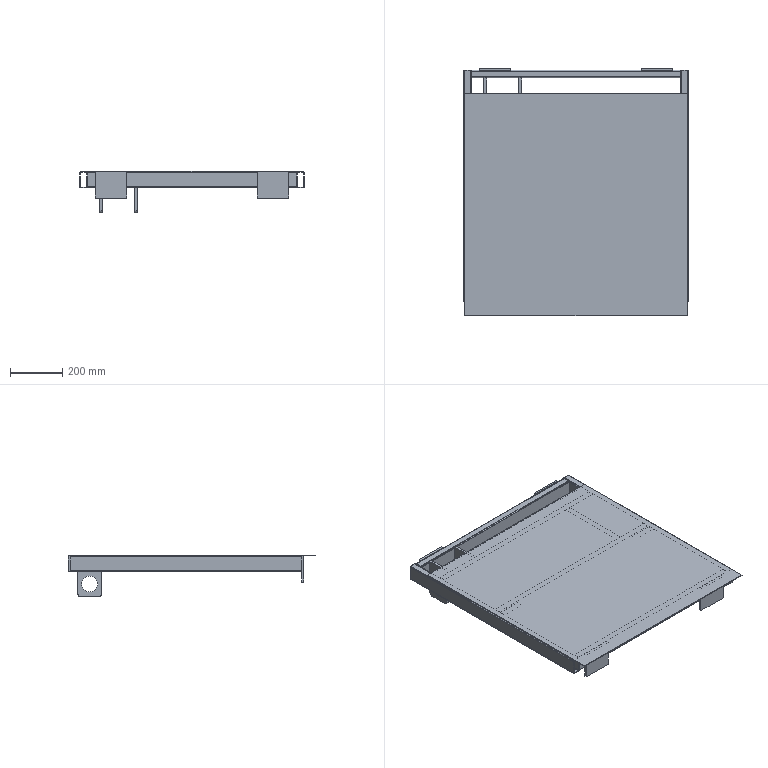Part | SolidWorks | features ICE 7, Split 3, WeldMemberFeat 3, LPattern 2, MirrorSolid 2, MoveFace 2, Fillet 1, WeldmentFeature 1 | 17 solids | 216 faces | box 860 x 948 x 160 mm | volume 4527013 mm3 | plane 134 | cylinder 82 | commonest cylinder face diameters 4 x36 8 x36 20 x4 61 x4 6 x2